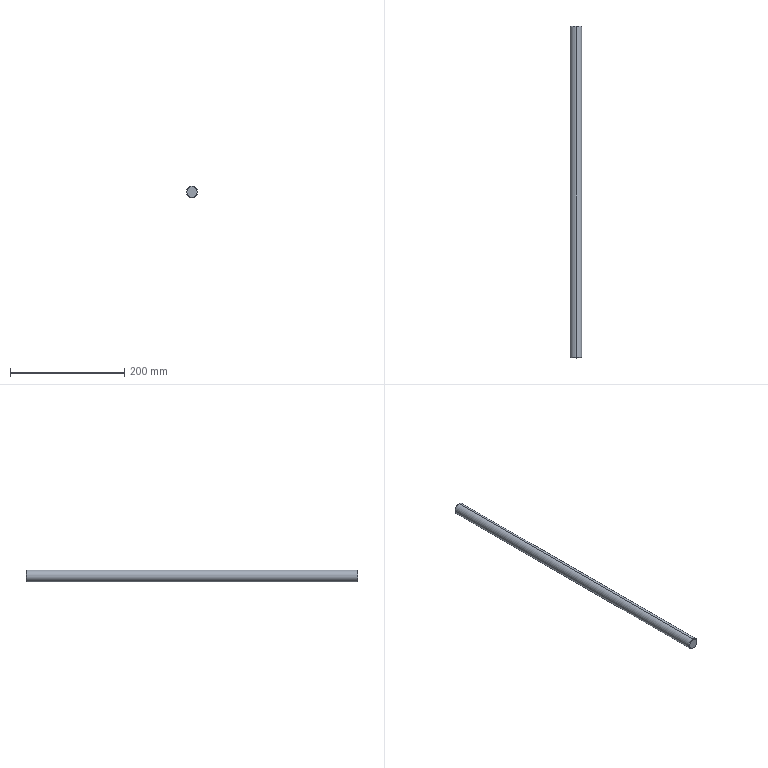Part | STEP file | 11-FG-S01711 | 1 solid | 12 faces | box 20 x 580 x 20 mm | volume 181847 mm3 | cone 6 | cylinder 4 | plane 2 | commonest cylinder face diameters 5 x2 20 x2
STEP:
#1=CARTESIAN_POINT('',(0.,580.,9.));
#2=VERTEX_POINT('',#1);
#3=CARTESIAN_POINT('',(0.,580.,-9.));
#4=VERTEX_POINT('',#3);
#5=CARTESIAN_POINT('',(0.,580.,0.));
#6=DIRECTION('',(0.,1.,0.));
#7=DIRECTION('',(0.,0.,1.));
#8=AXIS2_PLACEMENT_3D('',#5,#6,#7);
#9=CIRCLE('',#8,9.);
#10=EDGE_CURVE('',#2,#4,#9,.T.);
#11=ORIENTED_EDGE('',*,*,#10,.F.);
#12=CARTESIAN_POINT('',(0.,579.,10.));
#13=VERTEX_POINT('',#12);
#14=CARTESIAN_POINT('',(0.,580.,9.));
#15=DIRECTION('',(0.,-0.7071,0.7071));
#16=VECTOR('',#15,1000.);
#17=LINE('',#14,#16);
#18=EDGE_CURVE('',#2,#13,#17,.T.);
#19=ORIENTED_EDGE('',*,*,#18,.T.);
#20=CARTESIAN_POINT('',(0.,579.,-10.));
#21=VERTEX_POINT('',#20);
#22=CARTESIAN_POINT('',(0.,579.,0.));
#23=DIRECTION('',(0.,-1.,0.));
#24=DIRECTION('',(0.,0.,1.));
#25=AXIS2_PLACEMENT_3D('',#22,#23,#24);
#26=CIRCLE('',#25,10.);
#27=EDGE_CURVE('',#21,#13,#26,.T.);
#28=ORIENTED_EDGE('',*,*,#27,.F.);
#29=CARTESIAN_POINT('',(0.,580.,-9.));
#30=DIRECTION('',(0.,-0.7071,-0.7071));
#31=VECTOR('',#30,1000.);
#32=LINE('',#29,#31);
#33=EDGE_CURVE('',#4,#21,#32,.T.);
#34=ORIENTED_EDGE('',*,*,#33,.F.);
#35=EDGE_LOOP('',(#11,#19,#28,#34));
#36=FACE_OUTER_BOUND('',#35,.T.);
#37=CARTESIAN_POINT('',(0.,580.,0.));
#38=DIRECTION('',(0.,-1.,0.));
#39=DIRECTION('',(0.,0.,-1.));
#40=AXIS2_PLACEMENT_3D('',#37,#38,#39);
#41=CONICAL_SURFACE('',#40,9.,0.7854);
#42=ADVANCED_FACE('',(#36),#41,.T.);
#43=CARTESIAN_POINT('',(0.,0.,-9.));
#44=VERTEX_POINT('',#43);
#45=CARTESIAN_POINT('',(0.,0.,9.));
#46=VERTEX_POINT('',#45);
#47=CARTESIAN_POINT('',(0.,0.,0.));
#48=DIRECTION('',(0.,-1.,0.));
#49=DIRECTION('',(0.,0.,1.));
#50=AXIS2_PLACEMENT_3D('',#47,#48,#49);
#51=CIRCLE('',#50,9.);
#52=EDGE_CURVE('',#44,#46,#51,.T.);
#53=ORIENTED_EDGE('',*,*,#52,.F.);
#54=CARTESIAN_POINT('',(0.,1.,-10.));
#55=VERTEX_POINT('',#54);
#56=CARTESIAN_POINT('',(0.,1.,-10.));
#57=DIRECTION('',(0.,0.7071,-0.7071));
#58=VECTOR('',#57,1000.);
#59=LINE('',#56,#58);
#60=EDGE_CURVE('',#44,#55,#59,.T.);
#61=ORIENTED_EDGE('',*,*,#60,.T.);
#62=CARTESIAN_POINT('',(0.,1.,10.));
#63=VERTEX_POINT('',#62);
#64=CARTESIAN_POINT('',(0.,1.,0.));
#65=DIRECTION('',(0.,1.,0.));
#66=DIRECTION('',(0.,0.,1.));
#67=AXIS2_PLACEMENT_3D('',#64,#65,#66);
#68=CIRCLE('',#67,10.);
#69=EDGE_CURVE('',#63,#55,#68,.T.);
#70=ORIENTED_EDGE('',*,*,#69,.F.);
#71=CARTESIAN_POINT('',(0.,1.,10.));
#72=DIRECTION('',(0.,0.7071,0.7071));
#73=VECTOR('',#72,1000.);
#74=LINE('',#71,#73);
#75=EDGE_CURVE('',#46,#63,#74,.T.);
#76=ORIENTED_EDGE('',*,*,#75,.F.);
#77=EDGE_LOOP('',(#53,#61,#70,#76));
#78=FACE_OUTER_BOUND('',#77,.T.);
#79=CARTESIAN_POINT('',(0.,1.,0.));
#80=DIRECTION('',(0.,1.,0.));
#81=DIRECTION('',(0.,0.,1.));
#82=AXIS2_PLACEMENT_3D('',#79,#80,#81);
#83=CONICAL_SURFACE('',#82,10.,0.7854);
#84=ADVANCED_FACE('',(#78),#83,.T.);
#85=CARTESIAN_POINT('',(0.,565.,-2.5));
#86=VERTEX_POINT('',#85);
#87=CARTESIAN_POINT('',(0.,565.,2.5));
#88=VERTEX_POINT('',#87);
#89=CARTESIAN_POINT('',(0.,565.,0.));
#90=DIRECTION('',(0.,1.,0.));
#91=DIRECTION('',(0.,0.,1.));
#92=AXIS2_PLACEMENT_3D('',#89,#90,#91);
#93=CIRCLE('',#92,2.5);
#94=EDGE_CURVE('',#86,#88,#93,.T.);
#95=ORIENTED_EDGE('',*,*,#94,.F.);
#96=CARTESIAN_POINT('',(0.,580.,-2.5));
#97=VERTEX_POINT('',#96);
#98=CARTESIAN_POINT('',(0.,580.,-2.5));
#99=DIRECTION('',(0.,1.,0.));
#100=VECTOR('',#99,1000.);
#101=LINE('',#98,#100);
#102=EDGE_CURVE('',#86,#97,#101,.T.);
#103=ORIENTED_EDGE('',*,*,#102,.T.);
#104=CARTESIAN_POINT('',(0.,580.,2.5));
#105=VERTEX_POINT('',#104);
#106=CARTESIAN_POINT('',(0.,580.,0.));
#107=DIRECTION('',(0.,1.,0.));
#108=DIRECTION('',(0.,0.,1.));
#109=AXIS2_PLACEMENT_3D('',#106,#107,#108);
#110=CIRCLE('',#109,2.5);
#111=EDGE_CURVE('',#97,#105,#110,.T.);
#112=ORIENTED_EDGE('',*,*,#111,.T.);
#113=CARTESIAN_POINT('',(0.,580.,2.5));
#114=DIRECTION('',(0.,1.,0.));
#115=VECTOR('',#114,1000.);
#116=LINE('',#113,#115);
#117=EDGE_CURVE('',#88,#105,#116,.T.);
#118=ORIENTED_EDGE('',*,*,#117,.F.);
#119=EDGE_LOOP('',(#95,#103,#112,#118));
#120=FACE_OUTER_BOUND('',#119,.T.);
#121=CARTESIAN_POINT('',(0.,580.,0.));
#122=DIRECTION('',(0.,1.,0.));
#123=DIRECTION('',(0.,0.,1.));
#124=AXIS2_PLACEMENT_3D('',#121,#122,#123);
#125=CYLINDRICAL_SURFACE('',#124,2.5);
#126=ADVANCED_FACE('',(#120),#125,.F.);
#127=CARTESIAN_POINT('',(0.,563.498,0.));
#128=VERTEX_POINT('',#127);
#129=CARTESIAN_POINT('',(0.,565.,2.5));
#130=DIRECTION('',(0.,0.515,0.8572));
#131=VECTOR('',#130,1000.);
#132=LINE('',#129,#131);
#133=EDGE_CURVE('',#128,#88,#132,.T.);
#134=ORIENTED_EDGE('',*,*,#133,.F.);
#135=CARTESIAN_POINT('',(0.,565.,-2.5));
#136=DIRECTION('',(0.,0.515,-0.8572));
#137=VECTOR('',#136,1000.);
#138=LINE('',#135,#137);
#139=EDGE_CURVE('',#128,#86,#138,.T.);
#140=ORIENTED_EDGE('',*,*,#139,.T.);
#141=ORIENTED_EDGE('',*,*,#94,.T.);
#142=EDGE_LOOP('',(#134,#140,#141));
#143=FACE_OUTER_BOUND('',#142,.T.);
#144=CARTESIAN_POINT('',(0.,565.,0.));
#145=DIRECTION('',(0.,1.,0.));
#146=DIRECTION('',(0.,0.,1.));
#147=AXIS2_PLACEMENT_3D('',#144,#145,#146);
#148=CONICAL_SURFACE('',#147,2.5,1.03);
#149=ADVANCED_FACE('',(#143),#148,.F.);
#150=ORIENTED_EDGE('',*,*,#27,.T.);
#151=CARTESIAN_POINT('',(0.,580.,10.));
#152=DIRECTION('',(0.,-1.,0.));
#153=VECTOR('',#152,1000.);
#154=LINE('',#151,#153);
#155=EDGE_CURVE('',#13,#63,#154,.T.);
#156=ORIENTED_EDGE('',*,*,#155,.T.);
#157=ORIENTED_EDGE('',*,*,#69,.T.);
#158=CARTESIAN_POINT('',(0.,580.,-10.));
#159=DIRECTION('',(0.,-1.,0.));
#160=VECTOR('',#159,1000.);
#161=LINE('',#158,#160);
#162=EDGE_CURVE('',#21,#55,#161,.T.);
#163=ORIENTED_EDGE('',*,*,#162,.F.);
#164=EDGE_LOOP('',(#150,#156,#157,#163));
#165=FACE_OUTER_BOUND('',#164,.T.);
#166=CARTESIAN_POINT('',(0.,580.,0.));
#167=DIRECTION('',(0.,-1.,0.));
#168=DIRECTION('',(0.,0.,-1.));
#169=AXIS2_PLACEMENT_3D('',#166,#167,#168);
#170=CYLINDRICAL_SURFACE('',#169,10.);
#171=ADVANCED_FACE('',(#165),#170,.T.);
#172=ORIENTED_EDGE('',*,*,#155,.F.);
#173=CARTESIAN_POINT('',(0.,579.,0.));
#174=DIRECTION('',(0.,-1.,0.));
#175=DIRECTION('',(0.,0.,1.));
#176=AXIS2_PLACEMENT_3D('',#173,#174,#175);
#177=CIRCLE('',#176,10.);
#178=EDGE_CURVE('',#13,#21,#177,.T.);
#179=ORIENTED_EDGE('',*,*,#178,.T.);
#180=ORIENTED_EDGE('',*,*,#162,.T.);
#181=CARTESIAN_POINT('',(0.,1.,0.));
#182=DIRECTION('',(0.,1.,0.));
#183=DIRECTION('',(0.,0.,1.));
#184=AXIS2_PLACEMENT_3D('',#181,#182,#183);
#185=CIRCLE('',#184,10.);
#186=EDGE_CURVE('',#55,#63,#185,.T.);
#187=ORIENTED_EDGE('',*,*,#186,.T.);
#188=EDGE_LOOP('',(#172,#179,#180,#187));
#189=FACE_OUTER_BOUND('',#188,.T.);
#190=CARTESIAN_POINT('',(0.,580.,0.));
#191=DIRECTION('',(0.,-1.,0.));
#192=DIRECTION('',(0.,0.,-1.));
#193=AXIS2_PLACEMENT_3D('',#190,#191,#192);
#194=CYLINDRICAL_SURFACE('',#193,10.);
#195=ADVANCED_FACE('',(#189),#194,.T.);
#196=CARTESIAN_POINT('',(0.,580.,0.));
#197=DIRECTION('',(0.,1.,0.));
#198=DIRECTION('',(0.,0.,1.));
#199=AXIS2_PLACEMENT_3D('',#196,#197,#198);
#200=CIRCLE('',#199,9.);
#201=EDGE_CURVE('',#4,#2,#200,.T.);
#202=ORIENTED_EDGE('',*,*,#201,.T.);
#203=ORIENTED_EDGE('',*,*,#10,.T.);
#204=EDGE_LOOP('',(#202,#203));
#205=FACE_OUTER_BOUND('',#204,.T.);
#206=CARTESIAN_POINT('',(0.,580.,0.));
#207=DIRECTION('',(0.,1.,0.));
#208=DIRECTION('',(0.,0.,1.));
#209=AXIS2_PLACEMENT_3D('',#206,#207,#208);
#210=CIRCLE('',#209,2.5);
#211=EDGE_CURVE('',#105,#97,#210,.T.);
#212=ORIENTED_EDGE('',*,*,#211,.F.);
#213=ORIENTED_EDGE('',*,*,#111,.F.);
#214=EDGE_LOOP('',(#212,#213));
#215=FACE_BOUND('',#214,.T.);
#216=CARTESIAN_POINT('',(0.,580.,0.));
#217=DIRECTION('',(0.,1.,0.));
#218=DIRECTION('',(0.,0.,1.));
#219=AXIS2_PLACEMENT_3D('',#216,#217,#218);
#220=PLANE('',#219);
#221=ADVANCED_FACE('',(#205,#215),#220,.T.);
#222=CARTESIAN_POINT('',(0.,0.,0.));
#223=DIRECTION('',(0.,-1.,0.));
#224=DIRECTION('',(0.,0.,1.));
#225=AXIS2_PLACEMENT_3D('',#222,#223,#224);
#226=CIRCLE('',#225,9.);
#227=EDGE_CURVE('',#46,#44,#226,.T.);
#228=ORIENTED_EDGE('',*,*,#227,.T.);
#229=ORIENTED_EDGE('',*,*,#52,.T.);
#230=EDGE_LOOP('',(#228,#229));
#231=FACE_OUTER_BOUND('',#230,.T.);
#232=CARTESIAN_POINT('',(0.,0.,0.));
#233=DIRECTION('',(0.,1.,0.));
#234=DIRECTION('',(0.,0.,1.));
#235=AXIS2_PLACEMENT_3D('',#232,#233,#234);
#236=PLANE('',#235);
#237=ADVANCED_FACE('',(#231),#236,.F.);
#238=ORIENTED_EDGE('',*,*,#139,.F.);
#239=ORIENTED_EDGE('',*,*,#133,.T.);
#240=CARTESIAN_POINT('',(0.,565.,0.));
#241=DIRECTION('',(0.,1.,0.));
#242=DIRECTION('',(0.,0.,1.));
#243=AXIS2_PLACEMENT_3D('',#240,#241,#242);
#244=CIRCLE('',#243,2.5);
#245=EDGE_CURVE('',#88,#86,#244,.T.);
#246=ORIENTED_EDGE('',*,*,#245,.T.);
#247=EDGE_LOOP('',(#238,#239,#246));
#248=FACE_OUTER_BOUND('',#247,.T.);
#249=CARTESIAN_POINT('',(0.,565.,0.));
#250=DIRECTION('',(0.,1.,0.));
#251=DIRECTION('',(0.,0.,1.));
#252=AXIS2_PLACEMENT_3D('',#249,#250,#251);
#253=CONICAL_SURFACE('',#252,2.5,1.03);
#254=ADVANCED_FACE('',(#248),#253,.F.);
#255=ORIENTED_EDGE('',*,*,#102,.F.);
#256=ORIENTED_EDGE('',*,*,#245,.F.);
#257=ORIENTED_EDGE('',*,*,#117,.T.);
#258=ORIENTED_EDGE('',*,*,#211,.T.);
#259=EDGE_LOOP('',(#255,#256,#257,#258));
#260=FACE_OUTER_BOUND('',#259,.T.);
#261=CARTESIAN_POINT('',(0.,580.,0.));
#262=DIRECTION('',(0.,1.,0.));
#263=DIRECTION('',(0.,0.,1.));
#264=AXIS2_PLACEMENT_3D('',#261,#262,#263);
#265=CYLINDRICAL_SURFACE('',#264,2.5);
#266=ADVANCED_FACE('',(#260),#265,.F.);
#267=ORIENTED_EDGE('',*,*,#60,.F.);
#268=ORIENTED_EDGE('',*,*,#227,.F.);
#269=ORIENTED_EDGE('',*,*,#75,.T.);
#270=ORIENTED_EDGE('',*,*,#186,.F.);
#271=EDGE_LOOP('',(#267,#268,#269,#270));
#272=FACE_OUTER_BOUND('',#271,.T.);
#273=CARTESIAN_POINT('',(0.,1.,0.));
#274=DIRECTION('',(0.,1.,0.));
#275=DIRECTION('',(0.,0.,1.));
#276=AXIS2_PLACEMENT_3D('',#273,#274,#275);
#277=CONICAL_SURFACE('',#276,10.,0.7854);
#278=ADVANCED_FACE('',(#272),#277,.T.);
#279=ORIENTED_EDGE('',*,*,#18,.F.);
#280=ORIENTED_EDGE('',*,*,#201,.F.);
#281=ORIENTED_EDGE('',*,*,#33,.T.);
#282=ORIENTED_EDGE('',*,*,#178,.F.);
#283=EDGE_LOOP('',(#279,#280,#281,#282));
#284=FACE_OUTER_BOUND('',#283,.T.);
#285=CARTESIAN_POINT('',(0.,580.,0.));
#286=DIRECTION('',(0.,-1.,0.));
#287=DIRECTION('',(0.,0.,-1.));
#288=AXIS2_PLACEMENT_3D('',#285,#286,#287);
#289=CONICAL_SURFACE('',#288,9.,0.7854);
#290=ADVANCED_FACE('',(#284),#289,.T.);
#291=CLOSED_SHELL('',(#42,#84,#126,#149,#171,#195,#221,#237,#254,#266,#278,#290));
#292=MANIFOLD_SOLID_BREP('',#291);
#293=CARTESIAN_POINT('',(0.,0.,0.));
#294=DIRECTION('',(0.,0.,1.));
#295=DIRECTION('',(1.,0.,0.));
#296=AXIS2_PLACEMENT_3D('',#293,#294,#295);
#297=(LENGTH_UNIT()NAMED_UNIT(*)SI_UNIT(.MILLI.,.METRE.));
#298=UNCERTAINTY_MEASURE_WITH_UNIT(LENGTH_MEASURE(0.00001),#297,'','');
#299=(NAMED_UNIT(*)PLANE_ANGLE_UNIT()SI_UNIT($,.RADIAN.));
#300=(NAMED_UNIT(*)SI_UNIT($,.STERADIAN.)SOLID_ANGLE_UNIT());
#301=(GEOMETRIC_REPRESENTATION_CONTEXT(3)GLOBAL_UNCERTAINTY_ASSIGNED_CONTEXT((#298))GLOBAL_UNIT_ASSIGNED_CONTEXT((#297,#299,#300))REPRESENTATION_CONTEXT('',''));
#302=ADVANCED_BREP_SHAPE_REPRESENTATION('',(#292,#296),#301);